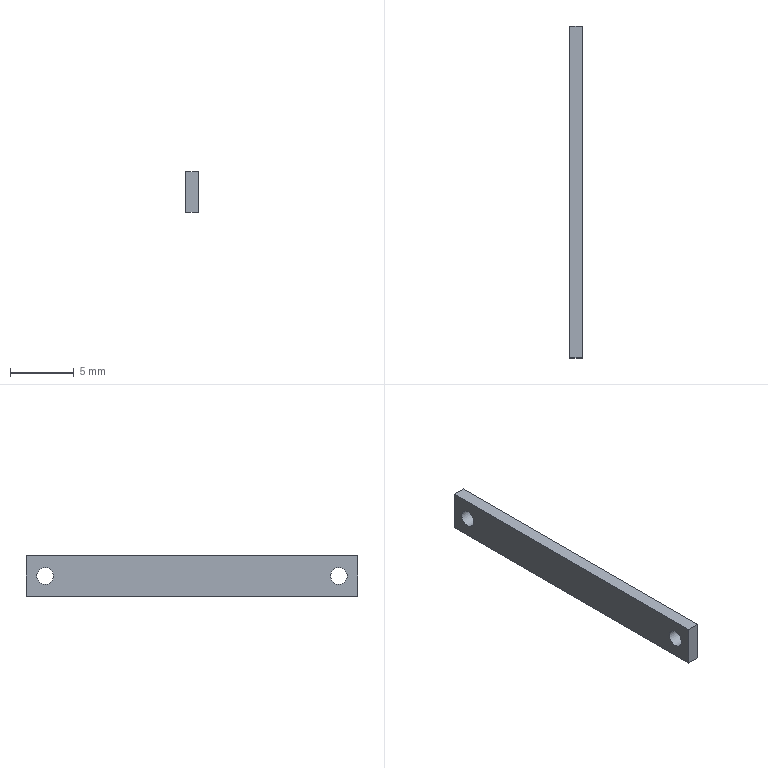Part | STEP file | Coupler coupling plate | 1 solid | 8 faces | box 1 x 26 x 3.21 mm | volume 80.805 mm3 | plane 6 | cylinder 2 | commonest cylinder face diameters 1.3 x2
STEP:
#1=CARTESIAN_POINT('',(0.,0.,0.));
#2=DIRECTION('',(0.,0.,1.));
#3=DIRECTION('',(1.,0.,0.));
#4=AXIS2_PLACEMENT_3D('',#1,#2,#3);
#5=CARTESIAN_POINT('',(12.25,-13.,1.605));
#6=VERTEX_POINT('',#5);
#7=CARTESIAN_POINT('',(12.25,-13.,-1.605));
#8=VERTEX_POINT('',#7);
#9=CARTESIAN_POINT('',(12.25,-13.,1.605));
#10=DIRECTION('',(0.,0.,-1.));
#11=VECTOR('',#10,1.);
#12=LINE('',#9,#11);
#13=CARTESIAN_POINT('',(11.25,-13.,1.605));
#14=DIRECTION('',(0.,-1.,0.));
#15=DIRECTION('',(0.,0.,-1.));
#16=AXIS2_PLACEMENT_3D('',#13,#14,#15);
#17=PLANE('',#16);
#18=CARTESIAN_POINT('',(0.,1.));
#19=DIRECTION('',(1.,0.));
#20=VECTOR('',#19,1.);
#21=LINE('',#18,#20);
#22=(GEOMETRIC_REPRESENTATION_CONTEXT(2)PARAMETRIC_REPRESENTATION_CONTEXT()REPRESENTATION_CONTEXT('',''));
#23=DEFINITIONAL_REPRESENTATION('',(#21),#22);
#24=PCURVE('',#17,#23);
#25=CARTESIAN_POINT('',(12.25,-11.5,0.));
#26=DIRECTION('',(-1.,0.,0.));
#27=DIRECTION('',(0.,0.,1.));
#28=AXIS2_PLACEMENT_3D('',#25,#26,#27);
#29=PLANE('',#28);
#30=CARTESIAN_POINT('',(1.605,-1.5));
#31=DIRECTION('',(-1.,0.));
#32=VECTOR('',#31,1.);
#33=LINE('',#30,#32);
#34=(GEOMETRIC_REPRESENTATION_CONTEXT(2)PARAMETRIC_REPRESENTATION_CONTEXT()REPRESENTATION_CONTEXT('',''));
#35=DEFINITIONAL_REPRESENTATION('',(#33),#34);
#36=PCURVE('',#29,#35);
#37=SURFACE_CURVE('',#12,(#24,#36),.PCURVE_S1.);
#38=EDGE_CURVE('',#6,#8,#37,.T.);
#39=ORIENTED_EDGE('',*,*,#38,.F.);
#40=CARTESIAN_POINT('',(11.25,-13.,1.605));
#41=VERTEX_POINT('',#40);
#42=CARTESIAN_POINT('',(11.25,-13.,1.605));
#43=DIRECTION('',(1.,0.,0.));
#44=VECTOR('',#43,1.);
#45=LINE('',#42,#44);
#46=CARTESIAN_POINT('',(0.,0.));
#47=DIRECTION('',(0.,1.));
#48=VECTOR('',#47,1.);
#49=LINE('',#46,#48);
#50=(GEOMETRIC_REPRESENTATION_CONTEXT(2)PARAMETRIC_REPRESENTATION_CONTEXT()REPRESENTATION_CONTEXT('',''));
#51=DEFINITIONAL_REPRESENTATION('',(#49),#50);
#52=PCURVE('',#17,#51);
#53=CARTESIAN_POINT('',(11.25,13.,1.605));
#54=DIRECTION('',(0.,0.,1.));
#55=DIRECTION('',(1.,0.,0.));
#56=AXIS2_PLACEMENT_3D('',#53,#54,#55);
#57=PLANE('',#56);
#58=CARTESIAN_POINT('',(0.,-26.));
#59=DIRECTION('',(1.,0.));
#60=VECTOR('',#59,1.);
#61=LINE('',#58,#60);
#62=(GEOMETRIC_REPRESENTATION_CONTEXT(2)PARAMETRIC_REPRESENTATION_CONTEXT()REPRESENTATION_CONTEXT('',''));
#63=DEFINITIONAL_REPRESENTATION('',(#61),#62);
#64=PCURVE('',#57,#63);
#65=SURFACE_CURVE('',#45,(#52,#64),.PCURVE_S1.);
#66=EDGE_CURVE('',#41,#6,#65,.T.);
#67=ORIENTED_EDGE('',*,*,#66,.F.);
#68=CARTESIAN_POINT('',(11.25,-13.,-1.605));
#69=VERTEX_POINT('',#68);
#70=CARTESIAN_POINT('',(11.25,-13.,1.605));
#71=DIRECTION('',(0.,0.,-1.));
#72=VECTOR('',#71,1.);
#73=LINE('',#70,#72);
#74=CARTESIAN_POINT('',(0.,0.));
#75=DIRECTION('',(1.,0.));
#76=VECTOR('',#75,1.);
#77=LINE('',#74,#76);
#78=(GEOMETRIC_REPRESENTATION_CONTEXT(2)PARAMETRIC_REPRESENTATION_CONTEXT()REPRESENTATION_CONTEXT('',''));
#79=DEFINITIONAL_REPRESENTATION('',(#77),#78);
#80=PCURVE('',#17,#79);
#81=CARTESIAN_POINT('',(11.25,-11.5,0.));
#82=DIRECTION('',(-1.,0.,0.));
#83=DIRECTION('',(0.,0.,1.));
#84=AXIS2_PLACEMENT_3D('',#81,#82,#83);
#85=PLANE('',#84);
#86=CARTESIAN_POINT('',(1.605,-1.5));
#87=DIRECTION('',(-1.,0.));
#88=VECTOR('',#87,1.);
#89=LINE('',#86,#88);
#90=(GEOMETRIC_REPRESENTATION_CONTEXT(2)PARAMETRIC_REPRESENTATION_CONTEXT()REPRESENTATION_CONTEXT('',''));
#91=DEFINITIONAL_REPRESENTATION('',(#89),#90);
#92=PCURVE('',#85,#91);
#93=SURFACE_CURVE('',#73,(#80,#92),.PCURVE_S1.);
#94=EDGE_CURVE('',#41,#69,#93,.T.);
#95=ORIENTED_EDGE('',*,*,#94,.T.);
#96=CARTESIAN_POINT('',(11.25,-13.,-1.605));
#97=DIRECTION('',(1.,0.,0.));
#98=VECTOR('',#97,1.);
#99=LINE('',#96,#98);
#100=CARTESIAN_POINT('',(3.21,0.));
#101=DIRECTION('',(0.,1.));
#102=VECTOR('',#101,1.);
#103=LINE('',#100,#102);
#104=(GEOMETRIC_REPRESENTATION_CONTEXT(2)PARAMETRIC_REPRESENTATION_CONTEXT()REPRESENTATION_CONTEXT('',''));
#105=DEFINITIONAL_REPRESENTATION('',(#103),#104);
#106=PCURVE('',#17,#105);
#107=CARTESIAN_POINT('',(11.25,-13.,-1.605));
#108=DIRECTION('',(0.,0.,-1.));
#109=DIRECTION('',(-1.,0.,0.));
#110=AXIS2_PLACEMENT_3D('',#107,#108,#109);
#111=PLANE('',#110);
#112=CARTESIAN_POINT('',(0.,0.));
#113=DIRECTION('',(-1.,0.));
#114=VECTOR('',#113,1.);
#115=LINE('',#112,#114);
#116=(GEOMETRIC_REPRESENTATION_CONTEXT(2)PARAMETRIC_REPRESENTATION_CONTEXT()REPRESENTATION_CONTEXT('',''));
#117=DEFINITIONAL_REPRESENTATION('',(#115),#116);
#118=PCURVE('',#111,#117);
#119=SURFACE_CURVE('',#99,(#106,#118),.PCURVE_S1.);
#120=EDGE_CURVE('',#69,#8,#119,.T.);
#121=ORIENTED_EDGE('',*,*,#120,.T.);
#122=EDGE_LOOP('',(#39,#67,#95,#121));
#123=FACE_BOUND('',#122,.T.);
#124=ADVANCED_FACE('',(#123),#17,.T.);
#125=CARTESIAN_POINT('',(12.25,13.,-1.605));
#126=VERTEX_POINT('',#125);
#127=CARTESIAN_POINT('',(12.25,-13.,-1.605));
#128=DIRECTION('',(0.,1.,0.));
#129=VECTOR('',#128,1.);
#130=LINE('',#127,#129);
#131=CARTESIAN_POINT('',(-1.,0.));
#132=DIRECTION('',(0.,1.));
#133=VECTOR('',#132,1.);
#134=LINE('',#131,#133);
#135=(GEOMETRIC_REPRESENTATION_CONTEXT(2)PARAMETRIC_REPRESENTATION_CONTEXT()REPRESENTATION_CONTEXT('',''));
#136=DEFINITIONAL_REPRESENTATION('',(#134),#135);
#137=PCURVE('',#111,#136);
#138=CARTESIAN_POINT('',(-1.605,-1.5));
#139=DIRECTION('',(0.,1.));
#140=VECTOR('',#139,1.);
#141=LINE('',#138,#140);
#142=(GEOMETRIC_REPRESENTATION_CONTEXT(2)PARAMETRIC_REPRESENTATION_CONTEXT()REPRESENTATION_CONTEXT('',''));
#143=DEFINITIONAL_REPRESENTATION('',(#141),#142);
#144=PCURVE('',#29,#143);
#145=SURFACE_CURVE('',#130,(#137,#144),.PCURVE_S1.);
#146=EDGE_CURVE('',#8,#126,#145,.T.);
#147=ORIENTED_EDGE('',*,*,#146,.F.);
#148=ORIENTED_EDGE('',*,*,#120,.F.);
#149=CARTESIAN_POINT('',(11.25,13.,-1.605));
#150=VERTEX_POINT('',#149);
#151=CARTESIAN_POINT('',(11.25,-13.,-1.605));
#152=DIRECTION('',(0.,1.,0.));
#153=VECTOR('',#152,1.);
#154=LINE('',#151,#153);
#155=CARTESIAN_POINT('',(0.,0.));
#156=DIRECTION('',(0.,1.));
#157=VECTOR('',#156,1.);
#158=LINE('',#155,#157);
#159=(GEOMETRIC_REPRESENTATION_CONTEXT(2)PARAMETRIC_REPRESENTATION_CONTEXT()REPRESENTATION_CONTEXT('',''));
#160=DEFINITIONAL_REPRESENTATION('',(#158),#159);
#161=PCURVE('',#111,#160);
#162=CARTESIAN_POINT('',(-1.605,-1.5));
#163=DIRECTION('',(0.,1.));
#164=VECTOR('',#163,1.);
#165=LINE('',#162,#164);
#166=(GEOMETRIC_REPRESENTATION_CONTEXT(2)PARAMETRIC_REPRESENTATION_CONTEXT()REPRESENTATION_CONTEXT('',''));
#167=DEFINITIONAL_REPRESENTATION('',(#165),#166);
#168=PCURVE('',#85,#167);
#169=SURFACE_CURVE('',#154,(#161,#168),.PCURVE_S1.);
#170=EDGE_CURVE('',#69,#150,#169,.T.);
#171=ORIENTED_EDGE('',*,*,#170,.T.);
#172=CARTESIAN_POINT('',(11.25,13.,-1.605));
#173=DIRECTION('',(1.,0.,0.));
#174=VECTOR('',#173,1.);
#175=LINE('',#172,#174);
#176=CARTESIAN_POINT('',(0.,26.));
#177=DIRECTION('',(-1.,0.));
#178=VECTOR('',#177,1.);
#179=LINE('',#176,#178);
#180=(GEOMETRIC_REPRESENTATION_CONTEXT(2)PARAMETRIC_REPRESENTATION_CONTEXT()REPRESENTATION_CONTEXT('',''));
#181=DEFINITIONAL_REPRESENTATION('',(#179),#180);
#182=PCURVE('',#111,#181);
#183=CARTESIAN_POINT('',(11.25,13.,-1.605));
#184=DIRECTION('',(0.,1.,0.));
#185=DIRECTION('',(0.,0.,1.));
#186=AXIS2_PLACEMENT_3D('',#183,#184,#185);
#187=PLANE('',#186);
#188=CARTESIAN_POINT('',(0.,0.));
#189=DIRECTION('',(0.,1.));
#190=VECTOR('',#189,1.);
#191=LINE('',#188,#190);
#192=(GEOMETRIC_REPRESENTATION_CONTEXT(2)PARAMETRIC_REPRESENTATION_CONTEXT()REPRESENTATION_CONTEXT('',''));
#193=DEFINITIONAL_REPRESENTATION('',(#191),#192);
#194=PCURVE('',#187,#193);
#195=SURFACE_CURVE('',#175,(#182,#194),.PCURVE_S1.);
#196=EDGE_CURVE('',#150,#126,#195,.T.);
#197=ORIENTED_EDGE('',*,*,#196,.T.);
#198=EDGE_LOOP('',(#147,#148,#171,#197));
#199=FACE_BOUND('',#198,.T.);
#200=ADVANCED_FACE('',(#199),#111,.T.);
#201=CARTESIAN_POINT('',(12.25,13.,1.605));
#202=VERTEX_POINT('',#201);
#203=CARTESIAN_POINT('',(12.25,13.,-1.605));
#204=DIRECTION('',(0.,0.,1.));
#205=VECTOR('',#204,1.);
#206=LINE('',#203,#205);
#207=CARTESIAN_POINT('',(0.,1.));
#208=DIRECTION('',(1.,0.));
#209=VECTOR('',#208,1.);
#210=LINE('',#207,#209);
#211=(GEOMETRIC_REPRESENTATION_CONTEXT(2)PARAMETRIC_REPRESENTATION_CONTEXT()REPRESENTATION_CONTEXT('',''));
#212=DEFINITIONAL_REPRESENTATION('',(#210),#211);
#213=PCURVE('',#187,#212);
#214=CARTESIAN_POINT('',(-1.605,24.5));
#215=DIRECTION('',(1.,0.));
#216=VECTOR('',#215,1.);
#217=LINE('',#214,#216);
#218=(GEOMETRIC_REPRESENTATION_CONTEXT(2)PARAMETRIC_REPRESENTATION_CONTEXT()REPRESENTATION_CONTEXT('',''));
#219=DEFINITIONAL_REPRESENTATION('',(#217),#218);
#220=PCURVE('',#29,#219);
#221=SURFACE_CURVE('',#206,(#213,#220),.PCURVE_S1.);
#222=EDGE_CURVE('',#126,#202,#221,.T.);
#223=ORIENTED_EDGE('',*,*,#222,.F.);
#224=ORIENTED_EDGE('',*,*,#196,.F.);
#225=CARTESIAN_POINT('',(11.25,13.,1.605));
#226=VERTEX_POINT('',#225);
#227=CARTESIAN_POINT('',(11.25,13.,-1.605));
#228=DIRECTION('',(0.,0.,1.));
#229=VECTOR('',#228,1.);
#230=LINE('',#227,#229);
#231=CARTESIAN_POINT('',(0.,0.));
#232=DIRECTION('',(1.,0.));
#233=VECTOR('',#232,1.);
#234=LINE('',#231,#233);
#235=(GEOMETRIC_REPRESENTATION_CONTEXT(2)PARAMETRIC_REPRESENTATION_CONTEXT()REPRESENTATION_CONTEXT('',''));
#236=DEFINITIONAL_REPRESENTATION('',(#234),#235);
#237=PCURVE('',#187,#236);
#238=CARTESIAN_POINT('',(-1.605,24.5));
#239=DIRECTION('',(1.,0.));
#240=VECTOR('',#239,1.);
#241=LINE('',#238,#240);
#242=(GEOMETRIC_REPRESENTATION_CONTEXT(2)PARAMETRIC_REPRESENTATION_CONTEXT()REPRESENTATION_CONTEXT('',''));
#243=DEFINITIONAL_REPRESENTATION('',(#241),#242);
#244=PCURVE('',#85,#243);
#245=SURFACE_CURVE('',#230,(#237,#244),.PCURVE_S1.);
#246=EDGE_CURVE('',#150,#226,#245,.T.);
#247=ORIENTED_EDGE('',*,*,#246,.T.);
#248=CARTESIAN_POINT('',(11.25,13.,1.605));
#249=DIRECTION('',(1.,0.,0.));
#250=VECTOR('',#249,1.);
#251=LINE('',#248,#250);
#252=CARTESIAN_POINT('',(3.21,0.));
#253=DIRECTION('',(0.,1.));
#254=VECTOR('',#253,1.);
#255=LINE('',#252,#254);
#256=(GEOMETRIC_REPRESENTATION_CONTEXT(2)PARAMETRIC_REPRESENTATION_CONTEXT()REPRESENTATION_CONTEXT('',''));
#257=DEFINITIONAL_REPRESENTATION('',(#255),#256);
#258=PCURVE('',#187,#257);
#259=CARTESIAN_POINT('',(0.,0.));
#260=DIRECTION('',(1.,0.));
#261=VECTOR('',#260,1.);
#262=LINE('',#259,#261);
#263=(GEOMETRIC_REPRESENTATION_CONTEXT(2)PARAMETRIC_REPRESENTATION_CONTEXT()REPRESENTATION_CONTEXT('',''));
#264=DEFINITIONAL_REPRESENTATION('',(#262),#263);
#265=PCURVE('',#57,#264);
#266=SURFACE_CURVE('',#251,(#258,#265),.PCURVE_S1.);
#267=EDGE_CURVE('',#226,#202,#266,.T.);
#268=ORIENTED_EDGE('',*,*,#267,.T.);
#269=EDGE_LOOP('',(#223,#224,#247,#268));
#270=FACE_BOUND('',#269,.T.);
#271=ADVANCED_FACE('',(#270),#187,.T.);
#272=CARTESIAN_POINT('',(12.25,-11.5,-0.65));
#273=VERTEX_POINT('',#272);
#274=CARTESIAN_POINT('',(12.25,-11.5,0.));
#275=DIRECTION('',(-1.,0.,0.));
#276=DIRECTION('',(0.,0.,-1.));
#277=AXIS2_PLACEMENT_3D('',#274,#275,#276);
#278=CIRCLE('',#277,0.65);
#279=CARTESIAN_POINT('',(11.25,-11.5,0.));
#280=DIRECTION('',(1.,0.,0.));
#281=DIRECTION('',(0.,0.,-1.));
#282=AXIS2_PLACEMENT_3D('',#279,#280,#281);
#283=CYLINDRICAL_SURFACE('',#282,0.65);
#284=CARTESIAN_POINT('',(6.283,1.));
#285=DIRECTION('',(-1.,0.));
#286=VECTOR('',#285,1.);
#287=LINE('',#284,#286);
#288=(GEOMETRIC_REPRESENTATION_CONTEXT(2)PARAMETRIC_REPRESENTATION_CONTEXT()REPRESENTATION_CONTEXT('',''));
#289=DEFINITIONAL_REPRESENTATION('',(#287),#288);
#290=PCURVE('',#283,#289);
#291=CARTESIAN_POINT('',(0.,0.));
#292=DIRECTION('',(-1.,0.));
#293=AXIS2_PLACEMENT_2D('',#291,#292);
#294=CIRCLE('',#293,0.65);
#295=(GEOMETRIC_REPRESENTATION_CONTEXT(2)PARAMETRIC_REPRESENTATION_CONTEXT()REPRESENTATION_CONTEXT('',''));
#296=DEFINITIONAL_REPRESENTATION('',(#294),#295);
#297=PCURVE('',#29,#296);
#298=SURFACE_CURVE('',#278,(#290,#297),.PCURVE_S1.);
#299=EDGE_CURVE('',#273,#273,#298,.T.);
#300=ORIENTED_EDGE('',*,*,#299,.T.);
#301=CARTESIAN_POINT('',(11.25,-11.5,-0.65));
#302=VERTEX_POINT('',#301);
#303=CARTESIAN_POINT('',(11.25,-11.5,-0.65));
#304=CARTESIAN_POINT('',(12.25,-11.5,-0.65));
#305=B_SPLINE_CURVE_WITH_KNOTS('',1,(#303,#304),.UNSPECIFIED.,.F.,.F.,(2,2),(0.,1.),.PIECEWISE_BEZIER_KNOTS.);
#306=CARTESIAN_POINT('',(0.,0.));
#307=DIRECTION('',(0.,1.));
#308=VECTOR('',#307,1.);
#309=LINE('',#306,#308);
#310=(GEOMETRIC_REPRESENTATION_CONTEXT(2)PARAMETRIC_REPRESENTATION_CONTEXT()REPRESENTATION_CONTEXT('',''));
#311=DEFINITIONAL_REPRESENTATION('',(#309),#310);
#312=PCURVE('',#283,#311);
#313=CARTESIAN_POINT('',(6.283,0.));
#314=DIRECTION('',(0.,1.));
#315=VECTOR('',#314,1.);
#316=LINE('',#313,#315);
#317=(GEOMETRIC_REPRESENTATION_CONTEXT(2)PARAMETRIC_REPRESENTATION_CONTEXT()REPRESENTATION_CONTEXT('',''));
#318=DEFINITIONAL_REPRESENTATION('',(#316),#317);
#319=PCURVE('',#283,#318);
#320=SEAM_CURVE('',#305,(#312,#319),.PCURVE_S1.);
#321=EDGE_CURVE('',#302,#273,#320,.T.);
#322=ORIENTED_EDGE('',*,*,#321,.F.);
#323=CARTESIAN_POINT('',(11.25,-11.5,0.));
#324=DIRECTION('',(-1.,0.,0.));
#325=DIRECTION('',(0.,0.,-1.));
#326=AXIS2_PLACEMENT_3D('',#323,#324,#325);
#327=CIRCLE('',#326,0.65);
#328=CARTESIAN_POINT('',(6.283,0.));
#329=DIRECTION('',(-1.,0.));
#330=VECTOR('',#329,1.);
#331=LINE('',#328,#330);
#332=(GEOMETRIC_REPRESENTATION_CONTEXT(2)PARAMETRIC_REPRESENTATION_CONTEXT()REPRESENTATION_CONTEXT('',''));
#333=DEFINITIONAL_REPRESENTATION('',(#331),#332);
#334=PCURVE('',#283,#333);
#335=CARTESIAN_POINT('',(0.,0.));
#336=DIRECTION('',(-1.,0.));
#337=AXIS2_PLACEMENT_2D('',#335,#336);
#338=CIRCLE('',#337,0.65);
#339=(GEOMETRIC_REPRESENTATION_CONTEXT(2)PARAMETRIC_REPRESENTATION_CONTEXT()REPRESENTATION_CONTEXT('',''));
#340=DEFINITIONAL_REPRESENTATION('',(#338),#339);
#341=PCURVE('',#85,#340);
#342=SURFACE_CURVE('',#327,(#334,#341),.PCURVE_S1.);
#343=EDGE_CURVE('',#302,#302,#342,.T.);
#344=ORIENTED_EDGE('',*,*,#343,.F.);
#345=ORIENTED_EDGE('',*,*,#321,.T.);
#346=EDGE_LOOP('',(#300,#322,#344,#345));
#347=FACE_BOUND('',#346,.F.);
#348=ADVANCED_FACE('',(#347),#283,.F.);
#349=CARTESIAN_POINT('',(12.25,13.,1.605));
#350=DIRECTION('',(0.,-1.,0.));
#351=VECTOR('',#350,1.);
#352=LINE('',#349,#351);
#353=CARTESIAN_POINT('',(1.,0.));
#354=DIRECTION('',(0.,-1.));
#355=VECTOR('',#354,1.);
#356=LINE('',#353,#355);
#357=(GEOMETRIC_REPRESENTATION_CONTEXT(2)PARAMETRIC_REPRESENTATION_CONTEXT()REPRESENTATION_CONTEXT('',''));
#358=DEFINITIONAL_REPRESENTATION('',(#356),#357);
#359=PCURVE('',#57,#358);
#360=CARTESIAN_POINT('',(1.605,24.5));
#361=DIRECTION('',(0.,-1.));
#362=VECTOR('',#361,1.);
#363=LINE('',#360,#362);
#364=(GEOMETRIC_REPRESENTATION_CONTEXT(2)PARAMETRIC_REPRESENTATION_CONTEXT()REPRESENTATION_CONTEXT('',''));
#365=DEFINITIONAL_REPRESENTATION('',(#363),#364);
#366=PCURVE('',#29,#365);
#367=SURFACE_CURVE('',#352,(#359,#366),.PCURVE_S1.);
#368=EDGE_CURVE('',#202,#6,#367,.T.);
#369=ORIENTED_EDGE('',*,*,#368,.F.);
#370=ORIENTED_EDGE('',*,*,#267,.F.);
#371=CARTESIAN_POINT('',(11.25,13.,1.605));
#372=DIRECTION('',(0.,-1.,0.));
#373=VECTOR('',#372,1.);
#374=LINE('',#371,#373);
#375=CARTESIAN_POINT('',(0.,0.));
#376=DIRECTION('',(0.,-1.));
#377=VECTOR('',#376,1.);
#378=LINE('',#375,#377);
#379=(GEOMETRIC_REPRESENTATION_CONTEXT(2)PARAMETRIC_REPRESENTATION_CONTEXT()REPRESENTATION_CONTEXT('',''));
#380=DEFINITIONAL_REPRESENTATION('',(#378),#379);
#381=PCURVE('',#57,#380);
#382=CARTESIAN_POINT('',(1.605,24.5));
#383=DIRECTION('',(0.,-1.));
#384=VECTOR('',#383,1.);
#385=LINE('',#382,#384);
#386=(GEOMETRIC_REPRESENTATION_CONTEXT(2)PARAMETRIC_REPRESENTATION_CONTEXT()REPRESENTATION_CONTEXT('',''));
#387=DEFINITIONAL_REPRESENTATION('',(#385),#386);
#388=PCURVE('',#85,#387);
#389=SURFACE_CURVE('',#374,(#381,#388),.PCURVE_S1.);
#390=EDGE_CURVE('',#226,#41,#389,.T.);
#391=ORIENTED_EDGE('',*,*,#390,.T.);
#392=ORIENTED_EDGE('',*,*,#66,.T.);
#393=EDGE_LOOP('',(#369,#370,#391,#392));
#394=FACE_BOUND('',#393,.T.);
#395=ADVANCED_FACE('',(#394),#57,.T.);
#396=CARTESIAN_POINT('',(12.25,11.5,-0.65));
#397=VERTEX_POINT('',#396);
#398=CARTESIAN_POINT('',(12.25,11.5,0.));
#399=DIRECTION('',(-1.,0.,0.));
#400=DIRECTION('',(0.,0.,-1.));
#401=AXIS2_PLACEMENT_3D('',#398,#399,#400);
#402=CIRCLE('',#401,0.65);
#403=CARTESIAN_POINT('',(11.25,11.5,0.));
#404=DIRECTION('',(1.,0.,0.));
#405=DIRECTION('',(0.,0.,-1.));
#406=AXIS2_PLACEMENT_3D('',#403,#404,#405);
#407=CYLINDRICAL_SURFACE('',#406,0.65);
#408=CARTESIAN_POINT('',(6.283,1.));
#409=DIRECTION('',(-1.,0.));
#410=VECTOR('',#409,1.);
#411=LINE('',#408,#410);
#412=(GEOMETRIC_REPRESENTATION_CONTEXT(2)PARAMETRIC_REPRESENTATION_CONTEXT()REPRESENTATION_CONTEXT('',''));
#413=DEFINITIONAL_REPRESENTATION('',(#411),#412);
#414=PCURVE('',#407,#413);
#415=CARTESIAN_POINT('',(0.,23.));
#416=DIRECTION('',(-1.,0.));
#417=AXIS2_PLACEMENT_2D('',#415,#416);
#418=CIRCLE('',#417,0.65);
#419=(GEOMETRIC_REPRESENTATION_CONTEXT(2)PARAMETRIC_REPRESENTATION_CONTEXT()REPRESENTATION_CONTEXT('',''));
#420=DEFINITIONAL_REPRESENTATION('',(#418),#419);
#421=PCURVE('',#29,#420);
#422=SURFACE_CURVE('',#402,(#414,#421),.PCURVE_S1.);
#423=EDGE_CURVE('',#397,#397,#422,.T.);
#424=ORIENTED_EDGE('',*,*,#423,.T.);
#425=CARTESIAN_POINT('',(11.25,11.5,-0.65));
#426=VERTEX_POINT('',#425);
#427=CARTESIAN_POINT('',(11.25,11.5,-0.65));
#428=CARTESIAN_POINT('',(12.25,11.5,-0.65));
#429=B_SPLINE_CURVE_WITH_KNOTS('',1,(#427,#428),.UNSPECIFIED.,.F.,.F.,(2,2),(0.,1.),.PIECEWISE_BEZIER_KNOTS.);
#430=CARTESIAN_POINT('',(0.,0.));
#431=DIRECTION('',(0.,1.));
#432=VECTOR('',#431,1.);
#433=LINE('',#430,#432);
#434=(GEOMETRIC_REPRESENTATION_CONTEXT(2)PARAMETRIC_REPRESENTATION_CONTEXT()REPRESENTATION_CONTEXT('',''));
#435=DEFINITIONAL_REPRESENTATION('',(#433),#434);
#436=PCURVE('',#407,#435);
#437=CARTESIAN_POINT('',(6.283,0.));
#438=DIRECTION('',(0.,1.));
#439=VECTOR('',#438,1.);
#440=LINE('',#437,#439);
#441=(GEOMETRIC_REPRESENTATION_CONTEXT(2)PARAMETRIC_REPRESENTATION_CONTEXT()REPRESENTATION_CONTEXT('',''));
#442=DEFINITIONAL_REPRESENTATION('',(#440),#441);
#443=PCURVE('',#407,#442);
#444=SEAM_CURVE('',#429,(#436,#443),.PCURVE_S1.);
#445=EDGE_CURVE('',#426,#397,#444,.T.);
#446=ORIENTED_EDGE('',*,*,#445,.F.);
#447=CARTESIAN_POINT('',(11.25,11.5,0.));
#448=DIRECTION('',(-1.,0.,0.));
#449=DIRECTION('',(0.,0.,-1.));
#450=AXIS2_PLACEMENT_3D('',#447,#448,#449);
#451=CIRCLE('',#450,0.65);
#452=CARTESIAN_POINT('',(6.283,0.));
#453=DIRECTION('',(-1.,0.));
#454=VECTOR('',#453,1.);
#455=LINE('',#452,#454);
#456=(GEOMETRIC_REPRESENTATION_CONTEXT(2)PARAMETRIC_REPRESENTATION_CONTEXT()REPRESENTATION_CONTEXT('',''));
#457=DEFINITIONAL_REPRESENTATION('',(#455),#456);
#458=PCURVE('',#407,#457);
#459=CARTESIAN_POINT('',(0.,23.));
#460=DIRECTION('',(-1.,0.));
#461=AXIS2_PLACEMENT_2D('',#459,#460);
#462=CIRCLE('',#461,0.65);
#463=(GEOMETRIC_REPRESENTATION_CONTEXT(2)PARAMETRIC_REPRESENTATION_CONTEXT()REPRESENTATION_CONTEXT('',''));
#464=DEFINITIONAL_REPRESENTATION('',(#462),#463);
#465=PCURVE('',#85,#464);
#466=SURFACE_CURVE('',#451,(#458,#465),.PCURVE_S1.);
#467=EDGE_CURVE('',#426,#426,#466,.T.);
#468=ORIENTED_EDGE('',*,*,#467,.F.);
#469=ORIENTED_EDGE('',*,*,#445,.T.);
#470=EDGE_LOOP('',(#424,#446,#468,#469));
#471=FACE_BOUND('',#470,.F.);
#472=ADVANCED_FACE('',(#471),#407,.F.);
#473=ORIENTED_EDGE('',*,*,#94,.F.);
#474=ORIENTED_EDGE('',*,*,#390,.F.);
#475=ORIENTED_EDGE('',*,*,#246,.F.);
#476=ORIENTED_EDGE('',*,*,#170,.F.);
#477=EDGE_LOOP('',(#473,#474,#475,#476));
#478=FACE_BOUND('',#477,.T.);
#479=ORIENTED_EDGE('',*,*,#343,.F.);
#480=EDGE_LOOP('',(#479));
#481=FACE_BOUND('',#480,.T.);
#482=ORIENTED_EDGE('',*,*,#467,.F.);
#483=EDGE_LOOP('',(#482));
#484=FACE_BOUND('',#483,.T.);
#485=ADVANCED_FACE('',(#478,#481,#484),#85,.T.);
#486=ORIENTED_EDGE('',*,*,#38,.T.);
#487=ORIENTED_EDGE('',*,*,#146,.T.);
#488=ORIENTED_EDGE('',*,*,#222,.T.);
#489=ORIENTED_EDGE('',*,*,#368,.T.);
#490=EDGE_LOOP('',(#486,#487,#488,#489));
#491=FACE_BOUND('',#490,.T.);
#492=ORIENTED_EDGE('',*,*,#299,.T.);
#493=EDGE_LOOP('',(#492));
#494=FACE_BOUND('',#493,.T.);
#495=ORIENTED_EDGE('',*,*,#423,.T.);
#496=EDGE_LOOP('',(#495));
#497=FACE_BOUND('',#496,.T.);
#498=ADVANCED_FACE('',(#491,#494,#497),#29,.F.);
#499=CLOSED_SHELL('',(#124,#200,#271,#348,#395,#472,#485,#498));
#500=MANIFOLD_SOLID_BREP('',#499);
#501=(LENGTH_UNIT()NAMED_UNIT(*)SI_UNIT(.MILLI.,.METRE.));
#502=UNCERTAINTY_MEASURE_WITH_UNIT(LENGTH_MEASURE(0.000002),#501,'','');
#503=(NAMED_UNIT(*)PLANE_ANGLE_UNIT()SI_UNIT($,.RADIAN.));
#504=(NAMED_UNIT(*)SI_UNIT($,.STERADIAN.)SOLID_ANGLE_UNIT());
#505=(GEOMETRIC_REPRESENTATION_CONTEXT(3)GLOBAL_UNCERTAINTY_ASSIGNED_CONTEXT((#502))GLOBAL_UNIT_ASSIGNED_CONTEXT((#501,#503,#504))REPRESENTATION_CONTEXT('',''));
#506=ADVANCED_BREP_SHAPE_REPRESENTATION('',(#4,#500),#505);